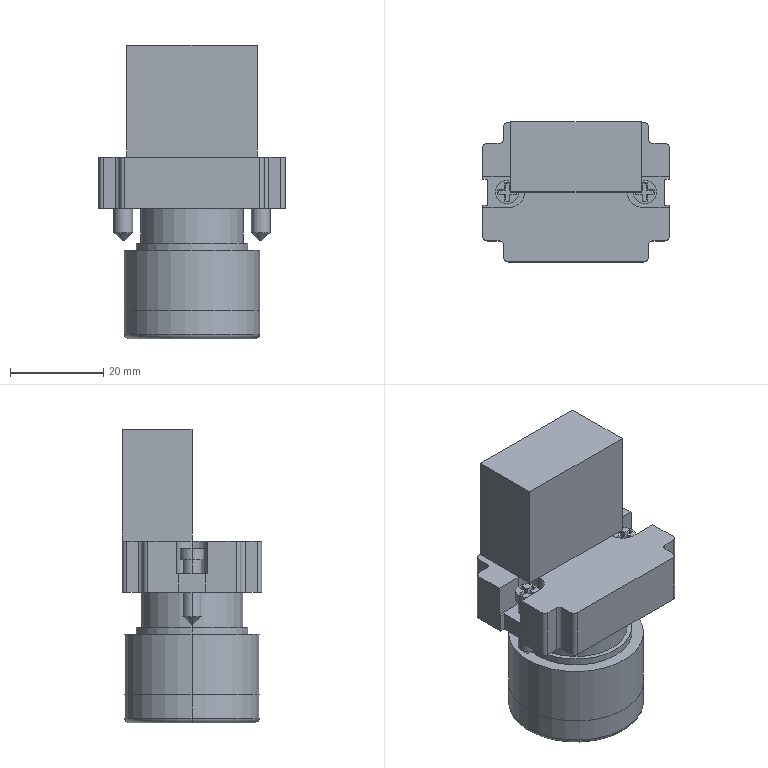Part | STEP file | Flat round head push button (yellow) | 3 solids | 111 faces | box 40 x 30 x 63 mm | volume 37927 mm3 | plane 70 | cylinder 35 | cone 4 | torus 2 | commonest cylinder face diameters 2 x12 4 x8 5 x4 29 x4 6.6 x3 22 x2